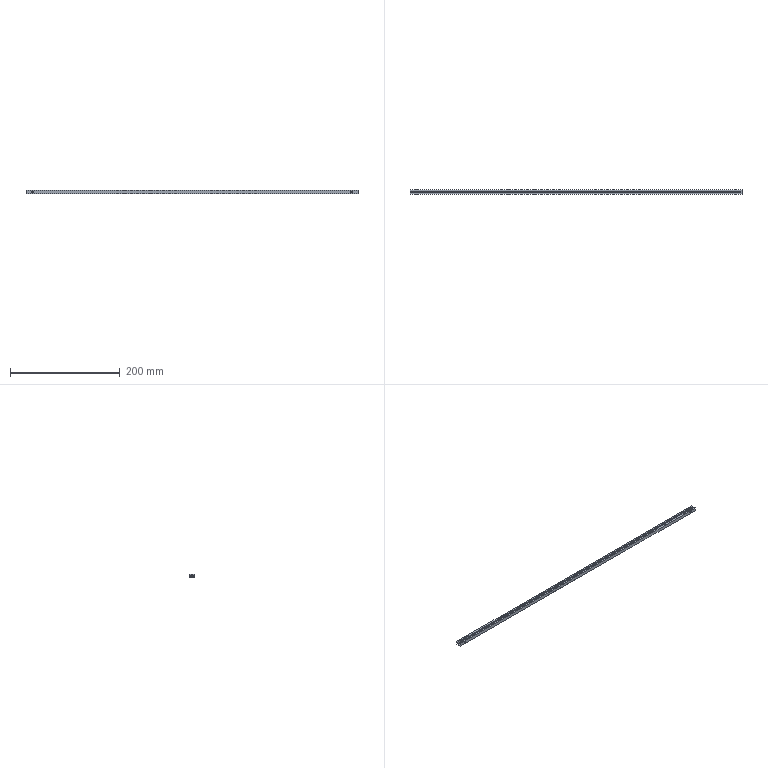Part | STEP file | SENAK3-X | 1 solid | 31 faces | box 606 x 9 x 6 mm | volume 19051 mm3 | plane 27 | cylinder 4 | commonest cylinder face diameters 3.5 x4